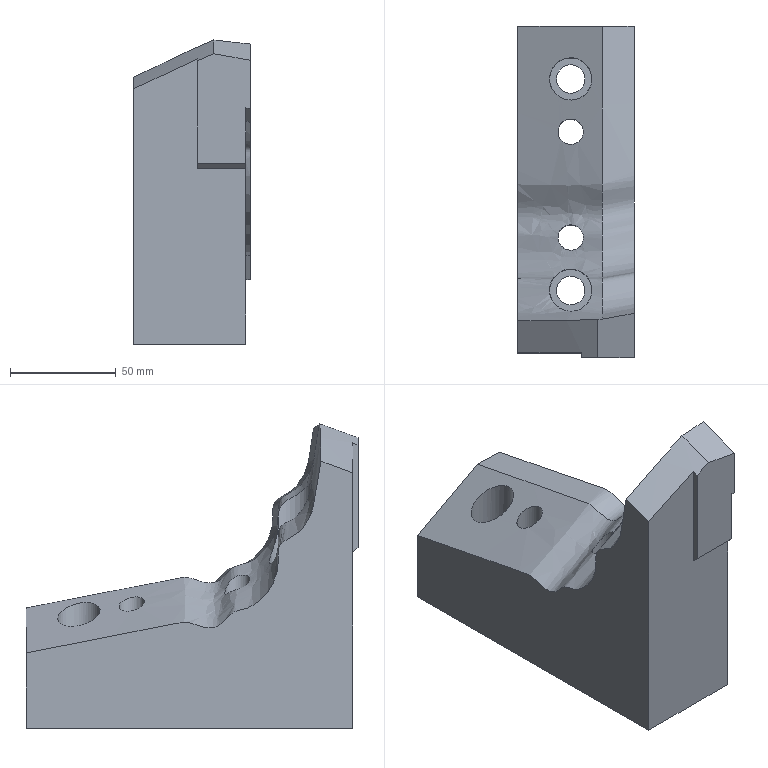Part | NX | features solid 2 | 1 solid | 23 faces | box 55 x 157 x 143.877 mm | volume 560575 mm3 | plane 9 | spline 8 | cylinder 6 | commonest cylinder face diameters 12 x2 13.5 x2 20 x2